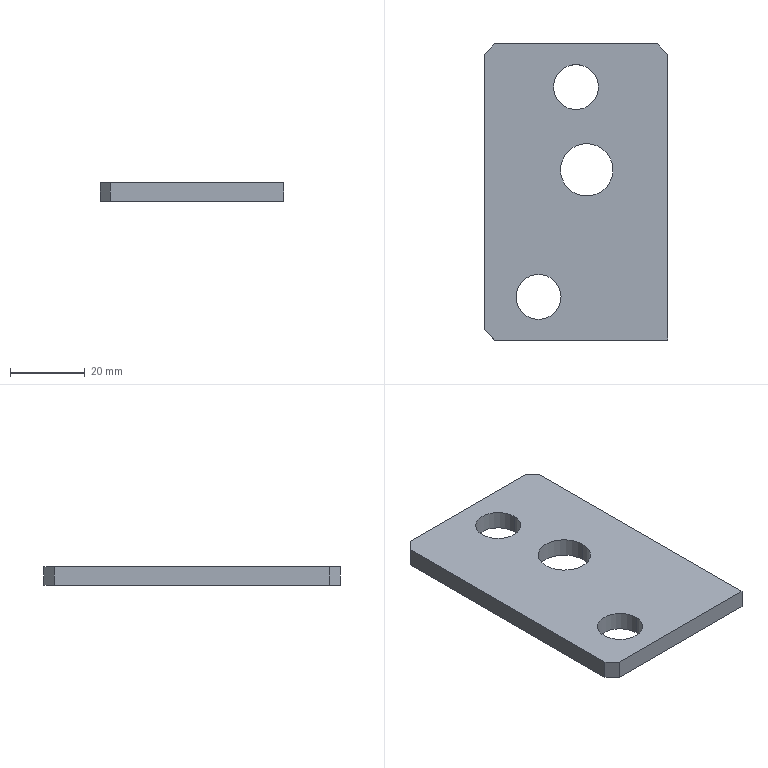Part | STEP file | 1_id646_x_t | 1 solid | 15 faces | box 49 x 79 x 5 mm | volume 17399 mm3 | plane 9 | cylinder 6 | commonest cylinder face diameters 12 x4 14 x2
STEP:
#1=CARTESIAN_POINT('',(0.,0.,0.));
#2=DIRECTION('',(0.,0.,1.));
#3=DIRECTION('',(1.,0.,0.));
#4=AXIS2_PLACEMENT_3D('',#1,#2,#3);
#5=CARTESIAN_POINT('',(168.943,211.1,-38.1));
#6=VERTEX_POINT('',#5);
#7=CARTESIAN_POINT('',(168.943,211.1,-43.1));
#8=VERTEX_POINT('',#7);
#9=CARTESIAN_POINT('',(168.943,211.1,-38.1));
#10=DIRECTION('',(0.,0.,-1.));
#11=VECTOR('',#10,1.);
#12=LINE('',#9,#11);
#13=CARTESIAN_POINT('',(149.775,211.1,-43.1));
#14=DIRECTION('',(0.,1.,0.));
#15=DIRECTION('',(0.,0.,-1.));
#16=AXIS2_PLACEMENT_3D('',#13,#14,#15);
#17=PLANE('',#16);
#18=CARTESIAN_POINT('',(-5.,-19.168));
#19=DIRECTION('',(1.,0.));
#20=VECTOR('',#19,1.);
#21=LINE('',#18,#20);
#22=(GEOMETRIC_REPRESENTATION_CONTEXT(2)PARAMETRIC_REPRESENTATION_CONTEXT()REPRESENTATION_CONTEXT('',''));
#23=DEFINITIONAL_REPRESENTATION('',(#21),#22);
#24=PCURVE('',#17,#23);
#25=CARTESIAN_POINT('',(173.659,206.384,-43.1));
#26=DIRECTION('',(-0.7071,-0.7071,0.));
#27=DIRECTION('',(-0.7071,0.7071,0.));
#28=AXIS2_PLACEMENT_3D('',#25,#26,#27);
#29=PLANE('',#28);
#30=CARTESIAN_POINT('',(6.67,-5.));
#31=DIRECTION('',(0.,1.));
#32=VECTOR('',#31,1.);
#33=LINE('',#30,#32);
#34=(GEOMETRIC_REPRESENTATION_CONTEXT(2)PARAMETRIC_REPRESENTATION_CONTEXT()REPRESENTATION_CONTEXT('',''));
#35=DEFINITIONAL_REPRESENTATION('',(#33),#34);
#36=PCURVE('',#29,#35);
#37=SURFACE_CURVE('',#12,(#24,#36),.PCURVE_S1.);
#38=EDGE_CURVE('',#6,#8,#37,.T.);
#39=ORIENTED_EDGE('',*,*,#38,.T.);
#40=CARTESIAN_POINT('',(125.357,211.1,-43.1));
#41=VERTEX_POINT('',#40);
#42=CARTESIAN_POINT('',(125.357,211.1,-43.1));
#43=DIRECTION('',(1.,0.,0.));
#44=VECTOR('',#43,1.);
#45=LINE('',#42,#44);
#46=CARTESIAN_POINT('',(0.,24.418));
#47=DIRECTION('',(0.,-1.));
#48=VECTOR('',#47,1.);
#49=LINE('',#46,#48);
#50=(GEOMETRIC_REPRESENTATION_CONTEXT(2)PARAMETRIC_REPRESENTATION_CONTEXT()REPRESENTATION_CONTEXT('',''));
#51=DEFINITIONAL_REPRESENTATION('',(#49),#50);
#52=PCURVE('',#17,#51);
#53=CARTESIAN_POINT('',(149.775,177.5,-43.1));
#54=DIRECTION('',(0.,0.,-1.));
#55=DIRECTION('',(-1.,0.,0.));
#56=AXIS2_PLACEMENT_3D('',#53,#54,#55);
#57=PLANE('',#56);
#58=CARTESIAN_POINT('',(24.418,33.6));
#59=DIRECTION('',(-1.,0.));
#60=VECTOR('',#59,1.);
#61=LINE('',#58,#60);
#62=(GEOMETRIC_REPRESENTATION_CONTEXT(2)PARAMETRIC_REPRESENTATION_CONTEXT()REPRESENTATION_CONTEXT('',''));
#63=DEFINITIONAL_REPRESENTATION('',(#61),#62);
#64=PCURVE('',#57,#63);
#65=SURFACE_CURVE('',#45,(#52,#64),.PCURVE_S1.);
#66=EDGE_CURVE('',#41,#8,#65,.T.);
#67=ORIENTED_EDGE('',*,*,#66,.F.);
#68=CARTESIAN_POINT('',(125.357,211.1,-38.1));
#69=VERTEX_POINT('',#68);
#70=CARTESIAN_POINT('',(125.357,211.1,-38.1));
#71=DIRECTION('',(0.,0.,-1.));
#72=VECTOR('',#71,1.);
#73=LINE('',#70,#72);
#74=CARTESIAN_POINT('',(-5.,24.418));
#75=DIRECTION('',(1.,0.));
#76=VECTOR('',#75,1.);
#77=LINE('',#74,#76);
#78=(GEOMETRIC_REPRESENTATION_CONTEXT(2)PARAMETRIC_REPRESENTATION_CONTEXT()REPRESENTATION_CONTEXT('',''));
#79=DEFINITIONAL_REPRESENTATION('',(#77),#78);
#80=PCURVE('',#17,#79);
#81=CARTESIAN_POINT('',(125.579,211.321,-43.1));
#82=DIRECTION('',(0.7071,-0.7071,0.));
#83=DIRECTION('',(-0.7071,-0.7071,0.));
#84=AXIS2_PLACEMENT_3D('',#81,#82,#83);
#85=PLANE('',#84);
#86=CARTESIAN_POINT('',(0.3132,-5.));
#87=DIRECTION('',(0.,1.));
#88=VECTOR('',#87,1.);
#89=LINE('',#86,#88);
#90=(GEOMETRIC_REPRESENTATION_CONTEXT(2)PARAMETRIC_REPRESENTATION_CONTEXT()REPRESENTATION_CONTEXT('',''));
#91=DEFINITIONAL_REPRESENTATION('',(#89),#90);
#92=PCURVE('',#85,#91);
#93=SURFACE_CURVE('',#73,(#80,#92),.PCURVE_S1.);
#94=EDGE_CURVE('',#69,#41,#93,.T.);
#95=ORIENTED_EDGE('',*,*,#94,.F.);
#96=CARTESIAN_POINT('',(125.357,211.1,-38.1));
#97=DIRECTION('',(1.,0.,0.));
#98=VECTOR('',#97,1.);
#99=LINE('',#96,#98);
#100=CARTESIAN_POINT('',(-5.,24.418));
#101=DIRECTION('',(0.,-1.));
#102=VECTOR('',#101,1.);
#103=LINE('',#100,#102);
#104=(GEOMETRIC_REPRESENTATION_CONTEXT(2)PARAMETRIC_REPRESENTATION_CONTEXT()REPRESENTATION_CONTEXT('',''));
#105=DEFINITIONAL_REPRESENTATION('',(#103),#104);
#106=PCURVE('',#17,#105);
#107=CARTESIAN_POINT('',(149.775,177.5,-38.1));
#108=DIRECTION('',(0.,0.,-1.));
#109=DIRECTION('',(-1.,0.,0.));
#110=AXIS2_PLACEMENT_3D('',#107,#108,#109);
#111=PLANE('',#110);
#112=CARTESIAN_POINT('',(24.418,33.6));
#113=DIRECTION('',(-1.,0.));
#114=VECTOR('',#113,1.);
#115=LINE('',#112,#114);
#116=(GEOMETRIC_REPRESENTATION_CONTEXT(2)PARAMETRIC_REPRESENTATION_CONTEXT()REPRESENTATION_CONTEXT('',''));
#117=DEFINITIONAL_REPRESENTATION('',(#115),#116);
#118=PCURVE('',#111,#117);
#119=SURFACE_CURVE('',#99,(#106,#118),.PCURVE_S1.);
#120=EDGE_CURVE('',#69,#6,#119,.T.);
#121=ORIENTED_EDGE('',*,*,#120,.T.);
#122=EDGE_LOOP('',(#39,#67,#95,#121));
#123=FACE_BOUND('',#122,.T.);
#124=ADVANCED_FACE('',(#123),#17,.T.);
#125=CARTESIAN_POINT('',(122.65,208.393,-38.1));
#126=VERTEX_POINT('',#125);
#127=CARTESIAN_POINT('',(125.357,211.1,-38.1));
#128=DIRECTION('',(-0.7071,-0.7071,0.));
#129=VECTOR('',#128,1.);
#130=LINE('',#127,#129);
#131=CARTESIAN_POINT('',(24.418,33.6));
#132=DIRECTION('',(0.7071,-0.7071));
#133=VECTOR('',#132,1.);
#134=LINE('',#131,#133);
#135=(GEOMETRIC_REPRESENTATION_CONTEXT(2)PARAMETRIC_REPRESENTATION_CONTEXT()REPRESENTATION_CONTEXT('',''));
#136=DEFINITIONAL_REPRESENTATION('',(#134),#135);
#137=PCURVE('',#111,#136);
#138=CARTESIAN_POINT('',(0.3132,-5.));
#139=DIRECTION('',(1.,0.));
#140=VECTOR('',#139,1.);
#141=LINE('',#138,#140);
#142=(GEOMETRIC_REPRESENTATION_CONTEXT(2)PARAMETRIC_REPRESENTATION_CONTEXT()REPRESENTATION_CONTEXT('',''));
#143=DEFINITIONAL_REPRESENTATION('',(#141),#142);
#144=PCURVE('',#85,#143);
#145=SURFACE_CURVE('',#130,(#137,#144),.PCURVE_S1.);
#146=EDGE_CURVE('',#69,#126,#145,.T.);
#147=ORIENTED_EDGE('',*,*,#146,.T.);
#148=CARTESIAN_POINT('',(122.65,134.807,-38.1));
#149=VERTEX_POINT('',#148);
#150=CARTESIAN_POINT('',(122.65,134.807,-38.1));
#151=DIRECTION('',(0.,1.,0.));
#152=VECTOR('',#151,1.);
#153=LINE('',#150,#152);
#154=CARTESIAN_POINT('',(27.125,-42.693));
#155=DIRECTION('',(0.,1.));
#156=VECTOR('',#155,1.);
#157=LINE('',#154,#156);
#158=(GEOMETRIC_REPRESENTATION_CONTEXT(2)PARAMETRIC_REPRESENTATION_CONTEXT()REPRESENTATION_CONTEXT('',''));
#159=DEFINITIONAL_REPRESENTATION('',(#157),#158);
#160=PCURVE('',#111,#159);
#161=CARTESIAN_POINT('',(122.65,173.5,-43.1));
#162=DIRECTION('',(-1.,0.,0.));
#163=DIRECTION('',(0.,0.,-1.));
#164=AXIS2_PLACEMENT_3D('',#161,#162,#163);
#165=PLANE('',#164);
#166=CARTESIAN_POINT('',(-5.,38.693));
#167=DIRECTION('',(0.,-1.));
#168=VECTOR('',#167,1.);
#169=LINE('',#166,#168);
#170=(GEOMETRIC_REPRESENTATION_CONTEXT(2)PARAMETRIC_REPRESENTATION_CONTEXT()REPRESENTATION_CONTEXT('',''));
#171=DEFINITIONAL_REPRESENTATION('',(#169),#170);
#172=PCURVE('',#165,#171);
#173=SURFACE_CURVE('',#153,(#160,#172),.PCURVE_S1.);
#174=EDGE_CURVE('',#149,#126,#173,.T.);
#175=ORIENTED_EDGE('',*,*,#174,.F.);
#176=CARTESIAN_POINT('',(125.357,132.1,-38.1));
#177=VERTEX_POINT('',#176);
#178=CARTESIAN_POINT('',(122.65,134.807,-38.1));
#179=DIRECTION('',(0.7071,-0.7071,0.));
#180=VECTOR('',#179,1.);
#181=LINE('',#178,#180);
#182=CARTESIAN_POINT('',(27.125,-42.693));
#183=DIRECTION('',(-0.7071,-0.7071));
#184=VECTOR('',#183,1.);
#185=LINE('',#182,#184);
#186=(GEOMETRIC_REPRESENTATION_CONTEXT(2)PARAMETRIC_REPRESENTATION_CONTEXT()REPRESENTATION_CONTEXT('',''));
#187=DEFINITIONAL_REPRESENTATION('',(#185),#186);
#188=PCURVE('',#111,#187);
#189=CARTESIAN_POINT('',(125.579,131.879,-43.1));
#190=DIRECTION('',(0.7071,0.7071,0.));
#191=DIRECTION('',(0.7071,-0.7071,0.));
#192=AXIS2_PLACEMENT_3D('',#189,#190,#191);
#193=PLANE('',#192);
#194=CARTESIAN_POINT('',(-4.142,-5.));
#195=DIRECTION('',(1.,0.));
#196=VECTOR('',#195,1.);
#197=LINE('',#194,#196);
#198=(GEOMETRIC_REPRESENTATION_CONTEXT(2)PARAMETRIC_REPRESENTATION_CONTEXT()REPRESENTATION_CONTEXT('',''));
#199=DEFINITIONAL_REPRESENTATION('',(#197),#198);
#200=PCURVE('',#193,#199);
#201=SURFACE_CURVE('',#181,(#188,#200),.PCURVE_S1.);
#202=EDGE_CURVE('',#149,#177,#201,.T.);
#203=ORIENTED_EDGE('',*,*,#202,.T.);
#204=CARTESIAN_POINT('',(171.65,132.1,-38.1));
#205=VERTEX_POINT('',#204);
#206=CARTESIAN_POINT('',(171.65,132.1,-38.1));
#207=DIRECTION('',(-1.,0.,0.));
#208=VECTOR('',#207,1.);
#209=LINE('',#206,#208);
#210=CARTESIAN_POINT('',(-21.875,-45.4));
#211=DIRECTION('',(1.,0.));
#212=VECTOR('',#211,1.);
#213=LINE('',#210,#212);
#214=(GEOMETRIC_REPRESENTATION_CONTEXT(2)PARAMETRIC_REPRESENTATION_CONTEXT()REPRESENTATION_CONTEXT('',''));
#215=DEFINITIONAL_REPRESENTATION('',(#213),#214);
#216=PCURVE('',#111,#215);
#217=CARTESIAN_POINT('',(149.775,132.1,-43.1));
#218=DIRECTION('',(0.,-1.,0.));
#219=DIRECTION('',(0.,0.,1.));
#220=AXIS2_PLACEMENT_3D('',#217,#218,#219);
#221=PLANE('',#220);
#222=CARTESIAN_POINT('',(5.,-21.875));
#223=DIRECTION('',(0.,1.));
#224=VECTOR('',#223,1.);
#225=LINE('',#222,#224);
#226=(GEOMETRIC_REPRESENTATION_CONTEXT(2)PARAMETRIC_REPRESENTATION_CONTEXT()REPRESENTATION_CONTEXT('',''));
#227=DEFINITIONAL_REPRESENTATION('',(#225),#226);
#228=PCURVE('',#221,#227);
#229=SURFACE_CURVE('',#209,(#216,#228),.PCURVE_S1.);
#230=EDGE_CURVE('',#205,#177,#229,.T.);
#231=ORIENTED_EDGE('',*,*,#230,.F.);
#232=CARTESIAN_POINT('',(171.65,208.393,-38.1));
#233=VERTEX_POINT('',#232);
#234=CARTESIAN_POINT('',(171.65,132.1,-38.1));
#235=DIRECTION('',(0.,1.,0.));
#236=VECTOR('',#235,1.);
#237=LINE('',#234,#236);
#238=CARTESIAN_POINT('',(-21.875,-45.4));
#239=DIRECTION('',(0.,1.));
#240=VECTOR('',#239,1.);
#241=LINE('',#238,#240);
#242=(GEOMETRIC_REPRESENTATION_CONTEXT(2)PARAMETRIC_REPRESENTATION_CONTEXT()REPRESENTATION_CONTEXT('',''));
#243=DEFINITIONAL_REPRESENTATION('',(#241),#242);
#244=PCURVE('',#111,#243);
#245=CARTESIAN_POINT('',(171.65,177.5,-43.1));
#246=DIRECTION('',(-1.,0.,0.));
#247=DIRECTION('',(0.,0.,-1.));
#248=AXIS2_PLACEMENT_3D('',#245,#246,#247);
#249=PLANE('',#248);
#250=CARTESIAN_POINT('',(-5.,45.4));
#251=DIRECTION('',(0.,-1.));
#252=VECTOR('',#251,1.);
#253=LINE('',#250,#252);
#254=(GEOMETRIC_REPRESENTATION_CONTEXT(2)PARAMETRIC_REPRESENTATION_CONTEXT()REPRESENTATION_CONTEXT('',''));
#255=DEFINITIONAL_REPRESENTATION('',(#253),#254);
#256=PCURVE('',#249,#255);
#257=SURFACE_CURVE('',#237,(#244,#256),.PCURVE_S1.);
#258=EDGE_CURVE('',#205,#233,#257,.T.);
#259=ORIENTED_EDGE('',*,*,#258,.T.);
#260=CARTESIAN_POINT('',(171.65,208.393,-38.1));
#261=DIRECTION('',(-0.7071,0.7071,0.));
#262=VECTOR('',#261,1.);
#263=LINE('',#260,#262);
#264=CARTESIAN_POINT('',(-21.875,30.893));
#265=DIRECTION('',(0.7071,0.7071));
#266=VECTOR('',#265,1.);
#267=LINE('',#264,#266);
#268=(GEOMETRIC_REPRESENTATION_CONTEXT(2)PARAMETRIC_REPRESENTATION_CONTEXT()REPRESENTATION_CONTEXT('',''));
#269=DEFINITIONAL_REPRESENTATION('',(#267),#268);
#270=PCURVE('',#111,#269);
#271=CARTESIAN_POINT('',(2.841,-5.));
#272=DIRECTION('',(1.,0.));
#273=VECTOR('',#272,1.);
#274=LINE('',#271,#273);
#275=(GEOMETRIC_REPRESENTATION_CONTEXT(2)PARAMETRIC_REPRESENTATION_CONTEXT()REPRESENTATION_CONTEXT('',''));
#276=DEFINITIONAL_REPRESENTATION('',(#274),#275);
#277=PCURVE('',#29,#276);
#278=SURFACE_CURVE('',#263,(#270,#277),.PCURVE_S1.);
#279=EDGE_CURVE('',#233,#6,#278,.T.);
#280=ORIENTED_EDGE('',*,*,#279,.T.);
#281=ORIENTED_EDGE('',*,*,#120,.F.);
#282=EDGE_LOOP('',(#147,#175,#203,#231,#259,#280,#281));
#283=FACE_BOUND('',#282,.T.);
#284=CARTESIAN_POINT('',(157.,177.5,-38.1));
#285=VERTEX_POINT('',#284);
#286=CARTESIAN_POINT('',(143.,177.5,-38.1));
#287=VERTEX_POINT('',#286);
#288=CARTESIAN_POINT('',(150.,177.5,-38.1));
#289=DIRECTION('',(0.,0.,-1.));
#290=DIRECTION('',(1.,0.,0.));
#291=AXIS2_PLACEMENT_3D('',#288,#289,#290);
#292=CIRCLE('',#291,7.);
#293=CARTESIAN_POINT('',(-0.225,-0.000000031));
#294=DIRECTION('',(-1.,0.));
#295=AXIS2_PLACEMENT_2D('',#293,#294);
#296=CIRCLE('',#295,7.);
#297=(GEOMETRIC_REPRESENTATION_CONTEXT(2)PARAMETRIC_REPRESENTATION_CONTEXT()REPRESENTATION_CONTEXT('',''));
#298=DEFINITIONAL_REPRESENTATION('',(#296),#297);
#299=PCURVE('',#111,#298);
#300=CARTESIAN_POINT('',(150.,177.5,-43.1));
#301=DIRECTION('',(0.,0.,1.));
#302=DIRECTION('',(-1.,0.,0.));
#303=AXIS2_PLACEMENT_3D('',#300,#301,#302);
#304=CYLINDRICAL_SURFACE('',#303,7.);
#305=CARTESIAN_POINT('',(3.142,5.));
#306=DIRECTION('',(-1.,0.));
#307=VECTOR('',#306,1.);
#308=LINE('',#305,#307);
#309=(GEOMETRIC_REPRESENTATION_CONTEXT(2)PARAMETRIC_REPRESENTATION_CONTEXT()REPRESENTATION_CONTEXT('',''));
#310=DEFINITIONAL_REPRESENTATION('',(#308),#309);
#311=PCURVE('',#304,#310);
#312=SURFACE_CURVE('',#292,(#299,#311),.PCURVE_S1.);
#313=EDGE_CURVE('',#285,#287,#312,.T.);
#314=ORIENTED_EDGE('',*,*,#313,.T.);
#315=CARTESIAN_POINT('',(150.,177.5,-38.1));
#316=DIRECTION('',(0.,0.,-1.));
#317=DIRECTION('',(-1.,0.,0.));
#318=AXIS2_PLACEMENT_3D('',#315,#316,#317);
#319=CIRCLE('',#318,7.);
#320=CARTESIAN_POINT('',(-0.225,-0.000000031));
#321=DIRECTION('',(1.,0.));
#322=AXIS2_PLACEMENT_2D('',#320,#321);
#323=CIRCLE('',#322,7.);
#324=(GEOMETRIC_REPRESENTATION_CONTEXT(2)PARAMETRIC_REPRESENTATION_CONTEXT()REPRESENTATION_CONTEXT('',''));
#325=DEFINITIONAL_REPRESENTATION('',(#323),#324);
#326=PCURVE('',#111,#325);
#327=CARTESIAN_POINT('',(150.,177.5,-43.1));
#328=DIRECTION('',(0.,0.,1.));
#329=DIRECTION('',(-1.,0.,0.));
#330=AXIS2_PLACEMENT_3D('',#327,#328,#329);
#331=CYLINDRICAL_SURFACE('',#330,7.);
#332=CARTESIAN_POINT('',(6.283,5.));
#333=DIRECTION('',(-1.,0.));
#334=VECTOR('',#333,1.);
#335=LINE('',#332,#334);
#336=(GEOMETRIC_REPRESENTATION_CONTEXT(2)PARAMETRIC_REPRESENTATION_CONTEXT()REPRESENTATION_CONTEXT('',''));
#337=DEFINITIONAL_REPRESENTATION('',(#335),#336);
#338=PCURVE('',#331,#337);
#339=SURFACE_CURVE('',#319,(#326,#338),.PCURVE_S1.);
#340=EDGE_CURVE('',#287,#285,#339,.T.);
#341=ORIENTED_EDGE('',*,*,#340,.T.);
#342=EDGE_LOOP('',(#314,#341));
#343=FACE_BOUND('',#342,.T.);
#344=CARTESIAN_POINT('',(143.15,143.6,-38.1));
#345=VERTEX_POINT('',#344);
#346=CARTESIAN_POINT('',(131.15,143.6,-38.1));
#347=VERTEX_POINT('',#346);
#348=CARTESIAN_POINT('',(137.15,143.6,-38.1));
#349=DIRECTION('',(0.,0.,-1.));
#350=DIRECTION('',(1.,0.,0.));
#351=AXIS2_PLACEMENT_3D('',#348,#349,#350);
#352=CIRCLE('',#351,6.);
#353=CARTESIAN_POINT('',(12.625,-33.9));
#354=DIRECTION('',(-1.,0.));
#355=AXIS2_PLACEMENT_2D('',#353,#354);
#356=CIRCLE('',#355,6.);
#357=(GEOMETRIC_REPRESENTATION_CONTEXT(2)PARAMETRIC_REPRESENTATION_CONTEXT()REPRESENTATION_CONTEXT('',''));
#358=DEFINITIONAL_REPRESENTATION('',(#356),#357);
#359=PCURVE('',#111,#358);
#360=CARTESIAN_POINT('',(137.15,143.6,-43.1));
#361=DIRECTION('',(0.,0.,1.));
#362=DIRECTION('',(-1.,0.,0.));
#363=AXIS2_PLACEMENT_3D('',#360,#361,#362);
#364=CYLINDRICAL_SURFACE('',#363,6.);
#365=CARTESIAN_POINT('',(3.142,5.));
#366=DIRECTION('',(-1.,0.));
#367=VECTOR('',#366,1.);
#368=LINE('',#365,#367);
#369=(GEOMETRIC_REPRESENTATION_CONTEXT(2)PARAMETRIC_REPRESENTATION_CONTEXT()REPRESENTATION_CONTEXT('',''));
#370=DEFINITIONAL_REPRESENTATION('',(#368),#369);
#371=PCURVE('',#364,#370);
#372=SURFACE_CURVE('',#352,(#359,#371),.PCURVE_S1.);
#373=EDGE_CURVE('',#345,#347,#372,.T.);
#374=ORIENTED_EDGE('',*,*,#373,.T.);
#375=CARTESIAN_POINT('',(137.15,143.6,-38.1));
#376=DIRECTION('',(0.,0.,-1.));
#377=DIRECTION('',(-1.,0.,0.));
#378=AXIS2_PLACEMENT_3D('',#375,#376,#377);
#379=CIRCLE('',#378,6.);
#380=CARTESIAN_POINT('',(12.625,-33.9));
#381=DIRECTION('',(1.,0.));
#382=AXIS2_PLACEMENT_2D('',#380,#381);
#383=CIRCLE('',#382,6.);
#384=(GEOMETRIC_REPRESENTATION_CONTEXT(2)PARAMETRIC_REPRESENTATION_CONTEXT()REPRESENTATION_CONTEXT('',''));
#385=DEFINITIONAL_REPRESENTATION('',(#383),#384);
#386=PCURVE('',#111,#385);
#387=CARTESIAN_POINT('',(137.15,143.6,-43.1));
#388=DIRECTION('',(0.,0.,1.));
#389=DIRECTION('',(-1.,0.,0.));
#390=AXIS2_PLACEMENT_3D('',#387,#388,#389);
#391=CYLINDRICAL_SURFACE('',#390,6.);
#392=CARTESIAN_POINT('',(6.283,5.));
#393=DIRECTION('',(-1.,0.));
#394=VECTOR('',#393,1.);
#395=LINE('',#392,#394);
#396=(GEOMETRIC_REPRESENTATION_CONTEXT(2)PARAMETRIC_REPRESENTATION_CONTEXT()REPRESENTATION_CONTEXT('',''));
#397=DEFINITIONAL_REPRESENTATION('',(#395),#396);
#398=PCURVE('',#391,#397);
#399=SURFACE_CURVE('',#379,(#386,#398),.PCURVE_S1.);
#400=EDGE_CURVE('',#347,#345,#399,.T.);
#401=ORIENTED_EDGE('',*,*,#400,.T.);
#402=EDGE_LOOP('',(#374,#401));
#403=FACE_BOUND('',#402,.T.);
#404=CARTESIAN_POINT('',(153.15,199.6,-38.1));
#405=VERTEX_POINT('',#404);
#406=CARTESIAN_POINT('',(141.15,199.6,-38.1));
#407=VERTEX_POINT('',#406);
#408=CARTESIAN_POINT('',(147.15,199.6,-38.1));
#409=DIRECTION('',(0.,0.,-1.));
#410=DIRECTION('',(1.,0.,0.));
#411=AXIS2_PLACEMENT_3D('',#408,#409,#410);
#412=CIRCLE('',#411,6.);
#413=CARTESIAN_POINT('',(2.625,22.1));
#414=DIRECTION('',(-1.,0.));
#415=AXIS2_PLACEMENT_2D('',#413,#414);
#416=CIRCLE('',#415,6.);
#417=(GEOMETRIC_REPRESENTATION_CONTEXT(2)PARAMETRIC_REPRESENTATION_CONTEXT()REPRESENTATION_CONTEXT('',''));
#418=DEFINITIONAL_REPRESENTATION('',(#416),#417);
#419=PCURVE('',#111,#418);
#420=CARTESIAN_POINT('',(147.15,199.6,-43.1));
#421=DIRECTION('',(0.,0.,1.));
#422=DIRECTION('',(-1.,0.,0.));
#423=AXIS2_PLACEMENT_3D('',#420,#421,#422);
#424=CYLINDRICAL_SURFACE('',#423,6.);
#425=CARTESIAN_POINT('',(3.142,5.));
#426=DIRECTION('',(-1.,0.));
#427=VECTOR('',#426,1.);
#428=LINE('',#425,#427);
#429=(GEOMETRIC_REPRESENTATION_CONTEXT(2)PARAMETRIC_REPRESENTATION_CONTEXT()REPRESENTATION_CONTEXT('',''));
#430=DEFINITIONAL_REPRESENTATION('',(#428),#429);
#431=PCURVE('',#424,#430);
#432=SURFACE_CURVE('',#412,(#419,#431),.PCURVE_S1.);
#433=EDGE_CURVE('',#405,#407,#432,.T.);
#434=ORIENTED_EDGE('',*,*,#433,.T.);
#435=CARTESIAN_POINT('',(147.15,199.6,-38.1));
#436=DIRECTION('',(0.,0.,-1.));
#437=DIRECTION('',(-1.,0.,0.));
#438=AXIS2_PLACEMENT_3D('',#435,#436,#437);
#439=CIRCLE('',#438,6.);
#440=CARTESIAN_POINT('',(2.625,22.1));
#441=DIRECTION('',(1.,0.));
#442=AXIS2_PLACEMENT_2D('',#440,#441);
#443=CIRCLE('',#442,6.);
#444=(GEOMETRIC_REPRESENTATION_CONTEXT(2)PARAMETRIC_REPRESENTATION_CONTEXT()REPRESENTATION_CONTEXT('',''));
#445=DEFINITIONAL_REPRESENTATION('',(#443),#444);
#446=PCURVE('',#111,#445);
#447=CARTESIAN_POINT('',(147.15,199.6,-43.1));
#448=DIRECTION('',(0.,0.,1.));
#449=DIRECTION('',(-1.,0.,0.));
#450=AXIS2_PLACEMENT_3D('',#447,#448,#449);
#451=CYLINDRICAL_SURFACE('',#450,6.);
#452=CARTESIAN_POINT('',(6.283,5.));
#453=DIRECTION('',(-1.,0.));
#454=VECTOR('',#453,1.);
#455=LINE('',#452,#454);
#456=(GEOMETRIC_REPRESENTATION_CONTEXT(2)PARAMETRIC_REPRESENTATION_CONTEXT()REPRESENTATION_CONTEXT('',''));
#457=DEFINITIONAL_REPRESENTATION('',(#455),#456);
#458=PCURVE('',#451,#457);
#459=SURFACE_CURVE('',#439,(#446,#458),.PCURVE_S1.);
#460=EDGE_CURVE('',#407,#405,#459,.T.);
#461=ORIENTED_EDGE('',*,*,#460,.T.);
#462=EDGE_LOOP('',(#434,#461));
#463=FACE_BOUND('',#462,.T.);
#464=ADVANCED_FACE('',(#283,#343,#403,#463),#111,.F.);
#465=CARTESIAN_POINT('',(157.,177.5,-43.1));
#466=VERTEX_POINT('',#465);
#467=CARTESIAN_POINT('',(143.,177.5,-43.1));
#468=VERTEX_POINT('',#467);
#469=CARTESIAN_POINT('',(150.,177.5,-43.1));
#470=DIRECTION('',(0.,0.,1.));
#471=DIRECTION('',(1.,0.,0.));
#472=AXIS2_PLACEMENT_3D('',#469,#470,#471);
#473=CIRCLE('',#472,7.);
#474=CARTESIAN_POINT('',(3.142,0.));
#475=DIRECTION('',(1.,0.));
#476=VECTOR('',#475,1.);
#477=LINE('',#474,#476);
#478=(GEOMETRIC_REPRESENTATION_CONTEXT(2)PARAMETRIC_REPRESENTATION_CONTEXT()REPRESENTATION_CONTEXT('',''));
#479=DEFINITIONAL_REPRESENTATION('',(#477),#478);
#480=PCURVE('',#331,#479);
#481=CARTESIAN_POINT('',(-7.225,-0.000000031));
#482=CARTESIAN_POINT('',(-7.225,12.124));
#483=CARTESIAN_POINT('',(3.275,6.062));
#484=CARTESIAN_POINT('',(13.775,-0.000000031));
#485=CARTESIAN_POINT('',(3.275,-6.062));
#486=CARTESIAN_POINT('',(-7.225,-12.124));
#487=CARTESIAN_POINT('',(-7.225,-0.000000031));
#488=(BOUNDED_CURVE()B_SPLINE_CURVE(2,(#481,#482,#483,#484,#485,#486,#487),.UNSPECIFIED.,.T.,.F.)B_SPLINE_CURVE_WITH_KNOTS((1,2,2,2,2,1),(-2.094,0.,2.094,4.189,6.283,8.378),.UNSPECIFIED.)CURVE()GEOMETRIC_REPRESENTATION_ITEM()RATIONAL_B_SPLINE_CURVE((1.,0.5,1.,0.5,1.,0.5,1.))REPRESENTATION_ITEM(''));
#489=(GEOMETRIC_REPRESENTATION_CONTEXT(2)PARAMETRIC_REPRESENTATION_CONTEXT()REPRESENTATION_CONTEXT('',''));
#490=DEFINITIONAL_REPRESENTATION('',(#488),#489);
#491=PCURVE('',#57,#490);
#492=SURFACE_CURVE('',#473,(#480,#491),.PCURVE_S1.);
#493=EDGE_CURVE('',#466,#468,#492,.T.);
#494=ORIENTED_EDGE('',*,*,#493,.T.);
#495=CARTESIAN_POINT('',(143.,177.5,-43.1));
#496=DIRECTION('',(0.,0.,1.));
#497=VECTOR('',#496,1.);
#498=LINE('',#495,#497);
#499=CARTESIAN_POINT('',(6.283,0.));
#500=DIRECTION('',(0.,1.));
#501=VECTOR('',#500,1.);
#502=LINE('',#499,#501);
#503=(GEOMETRIC_REPRESENTATION_CONTEXT(2)PARAMETRIC_REPRESENTATION_CONTEXT()REPRESENTATION_CONTEXT('',''));
#504=DEFINITIONAL_REPRESENTATION('',(#502),#503);
#505=PCURVE('',#331,#504);
#506=CARTESIAN_POINT('',(0.,0.));
#507=DIRECTION('',(0.,1.));
#508=VECTOR('',#507,1.);
#509=LINE('',#506,#508);
#510=(GEOMETRIC_REPRESENTATION_CONTEXT(2)PARAMETRIC_REPRESENTATION_CONTEXT()REPRESENTATION_CONTEXT('',''));
#511=DEFINITIONAL_REPRESENTATION('',(#509),#510);
#512=PCURVE('',#304,#511);
#513=SURFACE_CURVE('',#498,(#505,#512),.PCURVE_S1.);
#514=EDGE_CURVE('',#468,#287,#513,.T.);
#515=ORIENTED_EDGE('',*,*,#514,.T.);
#516=ORIENTED_EDGE('',*,*,#340,.T.);
#517=CARTESIAN_POINT('',(157.,177.5,-43.1));
#518=DIRECTION('',(0.,0.,-1.));
#519=VECTOR('',#518,1.);
#520=LINE('',#517,#519);
#521=CARTESIAN_POINT('',(3.142,0.));
#522=DIRECTION('',(0.,-1.));
#523=VECTOR('',#522,1.);
#524=LINE('',#521,#523);
#525=(GEOMETRIC_REPRESENTATION_CONTEXT(2)PARAMETRIC_REPRESENTATION_CONTEXT()REPRESENTATION_CONTEXT('',''));
#526=DEFINITIONAL_REPRESENTATION('',(#524),#525);
#527=PCURVE('',#331,#526);
#528=CARTESIAN_POINT('',(3.142,0.));
#529=DIRECTION('',(0.,-1.));
#530=VECTOR('',#529,1.);
#531=LINE('',#528,#530);
#532=(GEOMETRIC_REPRESENTATION_CONTEXT(2)PARAMETRIC_REPRESENTATION_CONTEXT()REPRESENTATION_CONTEXT('',''));
#533=DEFINITIONAL_REPRESENTATION('',(#531),#532);
#534=PCURVE('',#304,#533);
#535=SURFACE_CURVE('',#520,(#527,#534),.PCURVE_S1.);
#536=EDGE_CURVE('',#285,#466,#535,.T.);
#537=ORIENTED_EDGE('',*,*,#536,.T.);
#538=EDGE_LOOP('',(#494,#515,#516,#537));
#539=FACE_BOUND('',#538,.F.);
#540=ADVANCED_FACE('',(#539),#331,.F.);
#541=CARTESIAN_POINT('',(171.65,208.393,-43.1));
#542=VERTEX_POINT('',#541);
#543=CARTESIAN_POINT('',(168.943,211.1,-43.1));
#544=DIRECTION('',(0.7071,-0.7071,0.));
#545=VECTOR('',#544,1.);
#546=LINE('',#543,#545);
#547=CARTESIAN_POINT('',(-19.168,33.6));
#548=DIRECTION('',(-0.7071,-0.7071));
#549=VECTOR('',#548,1.);
#550=LINE('',#547,#549);
#551=(GEOMETRIC_REPRESENTATION_CONTEXT(2)PARAMETRIC_REPRESENTATION_CONTEXT()REPRESENTATION_CONTEXT('',''));
#552=DEFINITIONAL_REPRESENTATION('',(#550),#551);
#553=PCURVE('',#57,#552);
#554=CARTESIAN_POINT('',(6.67,0.));
#555=DIRECTION('',(-1.,0.));
#556=VECTOR('',#555,1.);
#557=LINE('',#554,#556);
#558=(GEOMETRIC_REPRESENTATION_CONTEXT(2)PARAMETRIC_REPRESENTATION_CONTEXT()REPRESENTATION_CONTEXT('',''));
#559=DEFINITIONAL_REPRESENTATION('',(#557),#558);
#560=PCURVE('',#29,#559);
#561=SURFACE_CURVE('',#546,(#553,#560),.PCURVE_S1.);
#562=EDGE_CURVE('',#8,#542,#561,.T.);
#563=ORIENTED_EDGE('',*,*,#562,.T.);
#564=CARTESIAN_POINT('',(171.65,132.1,-43.1));
#565=VERTEX_POINT('',#564);
#566=CARTESIAN_POINT('',(171.65,132.1,-43.1));
#567=DIRECTION('',(0.,1.,0.));
#568=VECTOR('',#567,1.);
#569=LINE('',#566,#568);
#570=CARTESIAN_POINT('',(-21.875,-45.4));
#571=DIRECTION('',(0.,1.));
#572=VECTOR('',#571,1.);
#573=LINE('',#570,#572);
#574=(GEOMETRIC_REPRESENTATION_CONTEXT(2)PARAMETRIC_REPRESENTATION_CONTEXT()REPRESENTATION_CONTEXT('',''));
#575=DEFINITIONAL_REPRESENTATION('',(#573),#574);
#576=PCURVE('',#57,#575);
#577=CARTESIAN_POINT('',(0.,45.4));
#578=DIRECTION('',(0.,-1.));
#579=VECTOR('',#578,1.);
#580=LINE('',#577,#579);
#581=(GEOMETRIC_REPRESENTATION_CONTEXT(2)PARAMETRIC_REPRESENTATION_CONTEXT()REPRESENTATION_CONTEXT('',''));
#582=DEFINITIONAL_REPRESENTATION('',(#580),#581);
#583=PCURVE('',#249,#582);
#584=SURFACE_CURVE('',#569,(#576,#583),.PCURVE_S1.);
#585=EDGE_CURVE('',#565,#542,#584,.T.);
#586=ORIENTED_EDGE('',*,*,#585,.F.);
#587=CARTESIAN_POINT('',(125.357,132.1,-43.1));
#588=VERTEX_POINT('',#587);
#589=CARTESIAN_POINT('',(171.65,132.1,-43.1));
#590=DIRECTION('',(-1.,0.,0.));
#591=VECTOR('',#590,1.);
#592=LINE('',#589,#591);
#593=CARTESIAN_POINT('',(-21.875,-45.4));
#594=DIRECTION('',(1.,0.));
#595=VECTOR('',#594,1.);
#596=LINE('',#593,#595);
#597=(GEOMETRIC_REPRESENTATION_CONTEXT(2)PARAMETRIC_REPRESENTATION_CONTEXT()REPRESENTATION_CONTEXT('',''));
#598=DEFINITIONAL_REPRESENTATION('',(#596),#597);
#599=PCURVE('',#57,#598);
#600=CARTESIAN_POINT('',(0.,-21.875));
#601=DIRECTION('',(0.,1.));
#602=VECTOR('',#601,1.);
#603=LINE('',#600,#602);
#604=(GEOMETRIC_REPRESENTATION_CONTEXT(2)PARAMETRIC_REPRESENTATION_CONTEXT()REPRESENTATION_CONTEXT('',''));
#605=DEFINITIONAL_REPRESENTATION('',(#603),#604);
#606=PCURVE('',#221,#605);
#607=SURFACE_CURVE('',#592,(#599,#606),.PCURVE_S1.);
#608=EDGE_CURVE('',#565,#588,#607,.T.);
#609=ORIENTED_EDGE('',*,*,#608,.T.);
#610=CARTESIAN_POINT('',(122.65,134.807,-43.1));
#611=VERTEX_POINT('',#610);
#612=CARTESIAN_POINT('',(125.357,132.1,-43.1));
#613=DIRECTION('',(-0.7071,0.7071,0.));
#614=VECTOR('',#613,1.);
#615=LINE('',#612,#614);
#616=CARTESIAN_POINT('',(24.418,-45.4));
#617=DIRECTION('',(0.7071,0.7071));
#618=VECTOR('',#617,1.);
#619=LINE('',#616,#618);
#620=(GEOMETRIC_REPRESENTATION_CONTEXT(2)PARAMETRIC_REPRESENTATION_CONTEXT()REPRESENTATION_CONTEXT('',''));
#621=DEFINITIONAL_REPRESENTATION('',(#619),#620);
#622=PCURVE('',#57,#621);
#623=CARTESIAN_POINT('',(-0.3132,0.));
#624=DIRECTION('',(-1.,0.));
#625=VECTOR('',#624,1.);
#626=LINE('',#623,#625);
#627=(GEOMETRIC_REPRESENTATION_CONTEXT(2)PARAMETRIC_REPRESENTATION_CONTEXT()REPRESENTATION_CONTEXT('',''));
#628=DEFINITIONAL_REPRESENTATION('',(#626),#627);
#629=PCURVE('',#193,#628);
#630=SURFACE_CURVE('',#615,(#622,#629),.PCURVE_S1.);
#631=EDGE_CURVE('',#588,#611,#630,.T.);
#632=ORIENTED_EDGE('',*,*,#631,.T.);
#633=CARTESIAN_POINT('',(122.65,208.393,-43.1));
#634=VERTEX_POINT('',#633);
#635=CARTESIAN_POINT('',(122.65,134.807,-43.1));
#636=DIRECTION('',(0.,1.,0.));
#637=VECTOR('',#636,1.);
#638=LINE('',#635,#637);
#639=CARTESIAN_POINT('',(27.125,-42.693));
#640=DIRECTION('',(0.,1.));
#641=VECTOR('',#640,1.);
#642=LINE('',#639,#641);
#643=(GEOMETRIC_REPRESENTATION_CONTEXT(2)PARAMETRIC_REPRESENTATION_CONTEXT()REPRESENTATION_CONTEXT('',''));
#644=DEFINITIONAL_REPRESENTATION('',(#642),#643);
#645=PCURVE('',#57,#644);
#646=CARTESIAN_POINT('',(0.,38.693));
#647=DIRECTION('',(0.,-1.));
#648=VECTOR('',#647,1.);
#649=LINE('',#646,#648);
#650=(GEOMETRIC_REPRESENTATION_CONTEXT(2)PARAMETRIC_REPRESENTATION_CONTEXT()REPRESENTATION_CONTEXT('',''));
#651=DEFINITIONAL_REPRESENTATION('',(#649),#650);
#652=PCURVE('',#165,#651);
#653=SURFACE_CURVE('',#638,(#645,#652),.PCURVE_S1.);
#654=EDGE_CURVE('',#611,#634,#653,.T.);
#655=ORIENTED_EDGE('',*,*,#654,.T.);
#656=CARTESIAN_POINT('',(122.65,208.393,-43.1));
#657=DIRECTION('',(0.7071,0.7071,0.));
#658=VECTOR('',#657,1.);
#659=LINE('',#656,#658);
#660=CARTESIAN_POINT('',(27.125,30.893));
#661=DIRECTION('',(-0.7071,0.7071));
#662=VECTOR('',#661,1.);
#663=LINE('',#660,#662);
#664=(GEOMETRIC_REPRESENTATION_CONTEXT(2)PARAMETRIC_REPRESENTATION_CONTEXT()REPRESENTATION_CONTEXT('',''));
#665=DEFINITIONAL_REPRESENTATION('',(#663),#664);
#666=PCURVE('',#57,#665);
#667=CARTESIAN_POINT('',(4.142,0.));
#668=DIRECTION('',(-1.,0.));
#669=VECTOR('',#668,1.);
#670=LINE('',#667,#669);
#671=(GEOMETRIC_REPRESENTATION_CONTEXT(2)PARAMETRIC_REPRESENTATION_CONTEXT()REPRESENTATION_CONTEXT('',''));
#672=DEFINITIONAL_REPRESENTATION('',(#670),#671);
#673=PCURVE('',#85,#672);
#674=SURFACE_CURVE('',#659,(#666,#673),.PCURVE_S1.);
#675=EDGE_CURVE('',#634,#41,#674,.T.);
#676=ORIENTED_EDGE('',*,*,#675,.T.);
#677=ORIENTED_EDGE('',*,*,#66,.T.);
#678=EDGE_LOOP('',(#563,#586,#609,#632,#655,#676,#677));
#679=FACE_BOUND('',#678,.T.);
#680=ORIENTED_EDGE('',*,*,#493,.T.);
#681=CARTESIAN_POINT('',(150.,177.5,-43.1));
#682=DIRECTION('',(0.,0.,1.));
#683=DIRECTION('',(-1.,0.,0.));
#684=AXIS2_PLACEMENT_3D('',#681,#682,#683);
#685=CIRCLE('',#684,7.);
#686=CARTESIAN_POINT('',(6.775,-0.000000031));
#687=CARTESIAN_POINT('',(6.775,-12.124));
#688=CARTESIAN_POINT('',(-3.725,-6.062));
#689=CARTESIAN_POINT('',(-14.225,-0.000000031));
#690=CARTESIAN_POINT('',(-3.725,6.062));
#691=CARTESIAN_POINT('',(6.775,12.124));
#692=CARTESIAN_POINT('',(6.775,-0.000000031));
#693=(BOUNDED_CURVE()B_SPLINE_CURVE(2,(#686,#687,#688,#689,#690,#691,#692),.UNSPECIFIED.,.T.,.F.)B_SPLINE_CURVE_WITH_KNOTS((1,2,2,2,2,1),(-2.094,0.,2.094,4.189,6.283,8.378),.UNSPECIFIED.)CURVE()GEOMETRIC_REPRESENTATION_ITEM()RATIONAL_B_SPLINE_CURVE((1.,0.5,1.,0.5,1.,0.5,1.))REPRESENTATION_ITEM(''));
#694=(GEOMETRIC_REPRESENTATION_CONTEXT(2)PARAMETRIC_REPRESENTATION_CONTEXT()REPRESENTATION_CONTEXT('',''));
#695=DEFINITIONAL_REPRESENTATION('',(#693),#694);
#696=PCURVE('',#57,#695);
#697=CARTESIAN_POINT('',(0.,0.));
#698=DIRECTION('',(1.,0.));
#699=VECTOR('',#698,1.);
#700=LINE('',#697,#699);
#701=(GEOMETRIC_REPRESENTATION_CONTEXT(2)PARAMETRIC_REPRESENTATION_CONTEXT()REPRESENTATION_CONTEXT('',''));
#702=DEFINITIONAL_REPRESENTATION('',(#700),#701);
#703=PCURVE('',#304,#702);
#704=SURFACE_CURVE('',#685,(#696,#703),.PCURVE_S1.);
#705=EDGE_CURVE('',#468,#466,#704,.T.);
#706=ORIENTED_EDGE('',*,*,#705,.T.);
#707=EDGE_LOOP('',(#680,#706));
#708=FACE_BOUND('',#707,.T.);
#709=CARTESIAN_POINT('',(143.15,143.6,-43.1));
#710=VERTEX_POINT('',#709);
#711=CARTESIAN_POINT('',(131.15,143.6,-43.1));
#712=VERTEX_POINT('',#711);
#713=CARTESIAN_POINT('',(137.15,143.6,-43.1));
#714=DIRECTION('',(0.,0.,1.));
#715=DIRECTION('',(1.,0.,0.));
#716=AXIS2_PLACEMENT_3D('',#713,#714,#715);
#717=CIRCLE('',#716,6.);
#718=CARTESIAN_POINT('',(6.625,-33.9));
#719=CARTESIAN_POINT('',(6.625,-23.508));
#720=CARTESIAN_POINT('',(15.625,-28.704));
#721=CARTESIAN_POINT('',(24.625,-33.9));
#722=CARTESIAN_POINT('',(15.625,-39.096));
#723=CARTESIAN_POINT('',(6.625,-44.292));
#724=CARTESIAN_POINT('',(6.625,-33.9));
#725=(BOUNDED_CURVE()B_SPLINE_CURVE(2,(#718,#719,#720,#721,#722,#723,#724),.UNSPECIFIED.,.T.,.F.)B_SPLINE_CURVE_WITH_KNOTS((1,2,2,2,2,1),(-2.094,0.,2.094,4.189,6.283,8.378),.UNSPECIFIED.)CURVE()GEOMETRIC_REPRESENTATION_ITEM()RATIONAL_B_SPLINE_CURVE((1.,0.5,1.,0.5,1.,0.5,1.))REPRESENTATION_ITEM(''));
#726=(GEOMETRIC_REPRESENTATION_CONTEXT(2)PARAMETRIC_REPRESENTATION_CONTEXT()REPRESENTATION_CONTEXT('',''));
#727=DEFINITIONAL_REPRESENTATION('',(#725),#726);
#728=PCURVE('',#57,#727);
#729=CARTESIAN_POINT('',(3.142,0.));
#730=DIRECTION('',(1.,0.));
#731=VECTOR('',#730,1.);
#732=LINE('',#729,#731);
#733=(GEOMETRIC_REPRESENTATION_CONTEXT(2)PARAMETRIC_REPRESENTATION_CONTEXT()REPRESENTATION_CONTEXT('',''));
#734=DEFINITIONAL_REPRESENTATION('',(#732),#733);
#735=PCURVE('',#391,#734);
#736=SURFACE_CURVE('',#717,(#728,#735),.PCURVE_S1.);
#737=EDGE_CURVE('',#710,#712,#736,.T.);
#738=ORIENTED_EDGE('',*,*,#737,.T.);
#739=CARTESIAN_POINT('',(137.15,143.6,-43.1));
#740=DIRECTION('',(0.,0.,1.));
#741=DIRECTION('',(-1.,0.,0.));
#742=AXIS2_PLACEMENT_3D('',#739,#740,#741);
#743=CIRCLE('',#742,6.);
#744=CARTESIAN_POINT('',(18.625,-33.9));
#745=CARTESIAN_POINT('',(18.625,-44.292));
#746=CARTESIAN_POINT('',(9.625,-39.096));
#747=CARTESIAN_POINT('',(0.625,-33.9));
#748=CARTESIAN_POINT('',(9.625,-28.704));
#749=CARTESIAN_POINT('',(18.625,-23.508));
#750=CARTESIAN_POINT('',(18.625,-33.9));
#751=(BOUNDED_CURVE()B_SPLINE_CURVE(2,(#744,#745,#746,#747,#748,#749,#750),.UNSPECIFIED.,.T.,.F.)B_SPLINE_CURVE_WITH_KNOTS((1,2,2,2,2,1),(-2.094,0.,2.094,4.189,6.283,8.378),.UNSPECIFIED.)CURVE()GEOMETRIC_REPRESENTATION_ITEM()RATIONAL_B_SPLINE_CURVE((1.,0.5,1.,0.5,1.,0.5,1.))REPRESENTATION_ITEM(''));
#752=(GEOMETRIC_REPRESENTATION_CONTEXT(2)PARAMETRIC_REPRESENTATION_CONTEXT()REPRESENTATION_CONTEXT('',''));
#753=DEFINITIONAL_REPRESENTATION('',(#751),#752);
#754=PCURVE('',#57,#753);
#755=CARTESIAN_POINT('',(0.,0.));
#756=DIRECTION('',(1.,0.));
#757=VECTOR('',#756,1.);
#758=LINE('',#755,#757);
#759=(GEOMETRIC_REPRESENTATION_CONTEXT(2)PARAMETRIC_REPRESENTATION_CONTEXT()REPRESENTATION_CONTEXT('',''));
#760=DEFINITIONAL_REPRESENTATION('',(#758),#759);
#761=PCURVE('',#364,#760);
#762=SURFACE_CURVE('',#743,(#754,#761),.PCURVE_S1.);
#763=EDGE_CURVE('',#712,#710,#762,.T.);
#764=ORIENTED_EDGE('',*,*,#763,.T.);
#765=EDGE_LOOP('',(#738,#764));
#766=FACE_BOUND('',#765,.T.);
#767=CARTESIAN_POINT('',(153.15,199.6,-43.1));
#768=VERTEX_POINT('',#767);
#769=CARTESIAN_POINT('',(141.15,199.6,-43.1));
#770=VERTEX_POINT('',#769);
#771=CARTESIAN_POINT('',(147.15,199.6,-43.1));
#772=DIRECTION('',(0.,0.,1.));
#773=DIRECTION('',(1.,0.,0.));
#774=AXIS2_PLACEMENT_3D('',#771,#772,#773);
#775=CIRCLE('',#774,6.);
#776=CARTESIAN_POINT('',(-3.375,22.1));
#777=CARTESIAN_POINT('',(-3.375,32.492));
#778=CARTESIAN_POINT('',(5.625,27.296));
#779=CARTESIAN_POINT('',(14.625,22.1));
#780=CARTESIAN_POINT('',(5.625,16.904));
#781=CARTESIAN_POINT('',(-3.375,11.708));
#782=CARTESIAN_POINT('',(-3.375,22.1));
#783=(BOUNDED_CURVE()B_SPLINE_CURVE(2,(#776,#777,#778,#779,#780,#781,#782),.UNSPECIFIED.,.T.,.F.)B_SPLINE_CURVE_WITH_KNOTS((1,2,2,2,2,1),(-2.094,0.,2.094,4.189,6.283,8.378),.UNSPECIFIED.)CURVE()GEOMETRIC_REPRESENTATION_ITEM()RATIONAL_B_SPLINE_CURVE((1.,0.5,1.,0.5,1.,0.5,1.))REPRESENTATION_ITEM(''));
#784=(GEOMETRIC_REPRESENTATION_CONTEXT(2)PARAMETRIC_REPRESENTATION_CONTEXT()REPRESENTATION_CONTEXT('',''));
#785=DEFINITIONAL_REPRESENTATION('',(#783),#784);
#786=PCURVE('',#57,#785);
#787=CARTESIAN_POINT('',(3.142,0.));
#788=DIRECTION('',(1.,0.));
#789=VECTOR('',#788,1.);
#790=LINE('',#787,#789);
#791=(GEOMETRIC_REPRESENTATION_CONTEXT(2)PARAMETRIC_REPRESENTATION_CONTEXT()REPRESENTATION_CONTEXT('',''));
#792=DEFINITIONAL_REPRESENTATION('',(#790),#791);
#793=PCURVE('',#451,#792);
#794=SURFACE_CURVE('',#775,(#786,#793),.PCURVE_S1.);
#795=EDGE_CURVE('',#768,#770,#794,.T.);
#796=ORIENTED_EDGE('',*,*,#795,.T.);
#797=CARTESIAN_POINT('',(147.15,199.6,-43.1));
#798=DIRECTION('',(0.,0.,1.));
#799=DIRECTION('',(-1.,0.,0.));
#800=AXIS2_PLACEMENT_3D('',#797,#798,#799);
#801=CIRCLE('',#800,6.);
#802=CARTESIAN_POINT('',(8.625,22.1));
#803=CARTESIAN_POINT('',(8.625,11.708));
#804=CARTESIAN_POINT('',(-0.375,16.904));
#805=CARTESIAN_POINT('',(-9.375,22.1));
#806=CARTESIAN_POINT('',(-0.375,27.296));
#807=CARTESIAN_POINT('',(8.625,32.492));
#808=CARTESIAN_POINT('',(8.625,22.1));
#809=(BOUNDED_CURVE()B_SPLINE_CURVE(2,(#802,#803,#804,#805,#806,#807,#808),.UNSPECIFIED.,.T.,.F.)B_SPLINE_CURVE_WITH_KNOTS((1,2,2,2,2,1),(-2.094,0.,2.094,4.189,6.283,8.378),.UNSPECIFIED.)CURVE()GEOMETRIC_REPRESENTATION_ITEM()RATIONAL_B_SPLINE_CURVE((1.,0.5,1.,0.5,1.,0.5,1.))REPRESENTATION_ITEM(''));
#810=(GEOMETRIC_REPRESENTATION_CONTEXT(2)PARAMETRIC_REPRESENTATION_CONTEXT()REPRESENTATION_CONTEXT('',''));
#811=DEFINITIONAL_REPRESENTATION('',(#809),#810);
#812=PCURVE('',#57,#811);
#813=CARTESIAN_POINT('',(0.,0.));
#814=DIRECTION('',(1.,0.));
#815=VECTOR('',#814,1.);
#816=LINE('',#813,#815);
#817=(GEOMETRIC_REPRESENTATION_CONTEXT(2)PARAMETRIC_REPRESENTATION_CONTEXT()REPRESENTATION_CONTEXT('',''));
#818=DEFINITIONAL_REPRESENTATION('',(#816),#817);
#819=PCURVE('',#424,#818);
#820=SURFACE_CURVE('',#801,(#812,#819),.PCURVE_S1.);
#821=EDGE_CURVE('',#770,#768,#820,.T.);
#822=ORIENTED_EDGE('',*,*,#821,.T.);
#823=EDGE_LOOP('',(#796,#822));
#824=FACE_BOUND('',#823,.T.);
#825=ADVANCED_FACE('',(#679,#708,#766,#824),#57,.T.);
#826=ORIENTED_EDGE('',*,*,#705,.T.);
#827=ORIENTED_EDGE('',*,*,#536,.F.);
#828=ORIENTED_EDGE('',*,*,#313,.T.);
#829=ORIENTED_EDGE('',*,*,#514,.F.);
#830=EDGE_LOOP('',(#826,#827,#828,#829));
#831=FACE_BOUND('',#830,.F.);
#832=ADVANCED_FACE('',(#831),#304,.F.);
#833=ORIENTED_EDGE('',*,*,#763,.T.);
#834=CARTESIAN_POINT('',(143.15,143.6,-43.1));
#835=DIRECTION('',(0.,0.,-1.));
#836=VECTOR('',#835,1.);
#837=LINE('',#834,#836);
#838=CARTESIAN_POINT('',(3.142,0.));
#839=DIRECTION('',(0.,-1.));
#840=VECTOR('',#839,1.);
#841=LINE('',#838,#840);
#842=(GEOMETRIC_REPRESENTATION_CONTEXT(2)PARAMETRIC_REPRESENTATION_CONTEXT()REPRESENTATION_CONTEXT('',''));
#843=DEFINITIONAL_REPRESENTATION('',(#841),#842);
#844=PCURVE('',#364,#843);
#845=CARTESIAN_POINT('',(3.142,0.));
#846=DIRECTION('',(0.,-1.));
#847=VECTOR('',#846,1.);
#848=LINE('',#845,#847);
#849=(GEOMETRIC_REPRESENTATION_CONTEXT(2)PARAMETRIC_REPRESENTATION_CONTEXT()REPRESENTATION_CONTEXT('',''));
#850=DEFINITIONAL_REPRESENTATION('',(#848),#849);
#851=PCURVE('',#391,#850);
#852=SURFACE_CURVE('',#837,(#844,#851),.PCURVE_S1.);
#853=EDGE_CURVE('',#345,#710,#852,.T.);
#854=ORIENTED_EDGE('',*,*,#853,.F.);
#855=ORIENTED_EDGE('',*,*,#373,.T.);
#856=CARTESIAN_POINT('',(131.15,143.6,-43.1));
#857=DIRECTION('',(0.,0.,1.));
#858=VECTOR('',#857,1.);
#859=LINE('',#856,#858);
#860=CARTESIAN_POINT('',(0.,0.));
#861=DIRECTION('',(0.,1.));
#862=VECTOR('',#861,1.);
#863=LINE('',#860,#862);
#864=(GEOMETRIC_REPRESENTATION_CONTEXT(2)PARAMETRIC_REPRESENTATION_CONTEXT()REPRESENTATION_CONTEXT('',''));
#865=DEFINITIONAL_REPRESENTATION('',(#863),#864);
#866=PCURVE('',#364,#865);
#867=CARTESIAN_POINT('',(6.283,0.));
#868=DIRECTION('',(0.,1.));
#869=VECTOR('',#868,1.);
#870=LINE('',#867,#869);
#871=(GEOMETRIC_REPRESENTATION_CONTEXT(2)PARAMETRIC_REPRESENTATION_CONTEXT()REPRESENTATION_CONTEXT('',''));
#872=DEFINITIONAL_REPRESENTATION('',(#870),#871);
#873=PCURVE('',#391,#872);
#874=SURFACE_CURVE('',#859,(#866,#873),.PCURVE_S1.);
#875=EDGE_CURVE('',#712,#347,#874,.T.);
#876=ORIENTED_EDGE('',*,*,#875,.F.);
#877=EDGE_LOOP('',(#833,#854,#855,#876));
#878=FACE_BOUND('',#877,.F.);
#879=ADVANCED_FACE('',(#878),#364,.F.);
#880=ORIENTED_EDGE('',*,*,#737,.T.);
#881=ORIENTED_EDGE('',*,*,#875,.T.);
#882=ORIENTED_EDGE('',*,*,#400,.T.);
#883=ORIENTED_EDGE('',*,*,#853,.T.);
#884=EDGE_LOOP('',(#880,#881,#882,#883));
#885=FACE_BOUND('',#884,.F.);
#886=ADVANCED_FACE('',(#885),#391,.F.);
#887=ORIENTED_EDGE('',*,*,#821,.T.);
#888=CARTESIAN_POINT('',(153.15,199.6,-43.1));
#889=DIRECTION('',(0.,0.,1.));
#890=VECTOR('',#889,1.);
#891=LINE('',#888,#890);
#892=CARTESIAN_POINT('',(3.142,0.));
#893=DIRECTION('',(0.,1.));
#894=VECTOR('',#893,1.);
#895=LINE('',#892,#894);
#896=(GEOMETRIC_REPRESENTATION_CONTEXT(2)PARAMETRIC_REPRESENTATION_CONTEXT()REPRESENTATION_CONTEXT('',''));
#897=DEFINITIONAL_REPRESENTATION('',(#895),#896);
#898=PCURVE('',#424,#897);
#899=CARTESIAN_POINT('',(3.142,0.));
#900=DIRECTION('',(0.,1.));
#901=VECTOR('',#900,1.);
#902=LINE('',#899,#901);
#903=(GEOMETRIC_REPRESENTATION_CONTEXT(2)PARAMETRIC_REPRESENTATION_CONTEXT()REPRESENTATION_CONTEXT('',''));
#904=DEFINITIONAL_REPRESENTATION('',(#902),#903);
#905=PCURVE('',#451,#904);
#906=SURFACE_CURVE('',#891,(#898,#905),.PCURVE_S1.);
#907=EDGE_CURVE('',#768,#405,#906,.T.);
#908=ORIENTED_EDGE('',*,*,#907,.T.);
#909=ORIENTED_EDGE('',*,*,#433,.T.);
#910=CARTESIAN_POINT('',(141.15,199.6,-43.1));
#911=DIRECTION('',(0.,0.,-1.));
#912=VECTOR('',#911,1.);
#913=LINE('',#910,#912);
#914=CARTESIAN_POINT('',(0.,0.));
#915=DIRECTION('',(0.,-1.));
#916=VECTOR('',#915,1.);
#917=LINE('',#914,#916);
#918=(GEOMETRIC_REPRESENTATION_CONTEXT(2)PARAMETRIC_REPRESENTATION_CONTEXT()REPRESENTATION_CONTEXT('',''));
#919=DEFINITIONAL_REPRESENTATION('',(#917),#918);
#920=PCURVE('',#424,#919);
#921=CARTESIAN_POINT('',(6.283,0.));
#922=DIRECTION('',(0.,-1.));
#923=VECTOR('',#922,1.);
#924=LINE('',#921,#923);
#925=(GEOMETRIC_REPRESENTATION_CONTEXT(2)PARAMETRIC_REPRESENTATION_CONTEXT()REPRESENTATION_CONTEXT('',''));
#926=DEFINITIONAL_REPRESENTATION('',(#924),#925);
#927=PCURVE('',#451,#926);
#928=SURFACE_CURVE('',#913,(#920,#927),.PCURVE_S1.);
#929=EDGE_CURVE('',#407,#770,#928,.T.);
#930=ORIENTED_EDGE('',*,*,#929,.T.);
#931=EDGE_LOOP('',(#887,#908,#909,#930));
#932=FACE_BOUND('',#931,.F.);
#933=ADVANCED_FACE('',(#932),#424,.F.);
#934=ORIENTED_EDGE('',*,*,#795,.T.);
#935=ORIENTED_EDGE('',*,*,#929,.F.);
#936=ORIENTED_EDGE('',*,*,#460,.T.);
#937=ORIENTED_EDGE('',*,*,#907,.F.);
#938=EDGE_LOOP('',(#934,#935,#936,#937));
#939=FACE_BOUND('',#938,.F.);
#940=ADVANCED_FACE('',(#939),#451,.F.);
#941=ORIENTED_EDGE('',*,*,#94,.T.);
#942=ORIENTED_EDGE('',*,*,#675,.F.);
#943=CARTESIAN_POINT('',(122.65,208.393,-38.1));
#944=DIRECTION('',(0.,0.,-1.));
#945=VECTOR('',#944,1.);
#946=LINE('',#943,#945);
#947=CARTESIAN_POINT('',(4.142,-5.));
#948=DIRECTION('',(0.,1.));
#949=VECTOR('',#948,1.);
#950=LINE('',#947,#949);
#951=(GEOMETRIC_REPRESENTATION_CONTEXT(2)PARAMETRIC_REPRESENTATION_CONTEXT()REPRESENTATION_CONTEXT('',''));
#952=DEFINITIONAL_REPRESENTATION('',(#950),#951);
#953=PCURVE('',#85,#952);
#954=CARTESIAN_POINT('',(-5.,-34.893));
#955=DIRECTION('',(1.,0.));
#956=VECTOR('',#955,1.);
#957=LINE('',#954,#956);
#958=(GEOMETRIC_REPRESENTATION_CONTEXT(2)PARAMETRIC_REPRESENTATION_CONTEXT()REPRESENTATION_CONTEXT('',''));
#959=DEFINITIONAL_REPRESENTATION('',(#957),#958);
#960=PCURVE('',#165,#959);
#961=SURFACE_CURVE('',#946,(#953,#960),.PCURVE_S1.);
#962=EDGE_CURVE('',#126,#634,#961,.T.);
#963=ORIENTED_EDGE('',*,*,#962,.F.);
#964=ORIENTED_EDGE('',*,*,#146,.F.);
#965=EDGE_LOOP('',(#941,#942,#963,#964));
#966=FACE_BOUND('',#965,.T.);
#967=ADVANCED_FACE('',(#966),#85,.F.);
#968=ORIENTED_EDGE('',*,*,#962,.T.);
#969=ORIENTED_EDGE('',*,*,#654,.F.);
#970=CARTESIAN_POINT('',(122.65,134.807,-38.1));
#971=DIRECTION('',(0.,0.,-1.));
#972=VECTOR('',#971,1.);
#973=LINE('',#970,#972);
#974=CARTESIAN_POINT('',(-5.,38.693));
#975=DIRECTION('',(1.,0.));
#976=VECTOR('',#975,1.);
#977=LINE('',#974,#976);
#978=(GEOMETRIC_REPRESENTATION_CONTEXT(2)PARAMETRIC_REPRESENTATION_CONTEXT()REPRESENTATION_CONTEXT('',''));
#979=DEFINITIONAL_REPRESENTATION('',(#977),#978);
#980=PCURVE('',#165,#979);
#981=CARTESIAN_POINT('',(-4.142,-5.));
#982=DIRECTION('',(0.,1.));
#983=VECTOR('',#982,1.);
#984=LINE('',#981,#983);
#985=(GEOMETRIC_REPRESENTATION_CONTEXT(2)PARAMETRIC_REPRESENTATION_CONTEXT()REPRESENTATION_CONTEXT('',''));
#986=DEFINITIONAL_REPRESENTATION('',(#984),#985);
#987=PCURVE('',#193,#986);
#988=SURFACE_CURVE('',#973,(#980,#987),.PCURVE_S1.);
#989=EDGE_CURVE('',#149,#611,#988,.T.);
#990=ORIENTED_EDGE('',*,*,#989,.F.);
#991=ORIENTED_EDGE('',*,*,#174,.T.);
#992=EDGE_LOOP('',(#968,#969,#990,#991));
#993=FACE_BOUND('',#992,.T.);
#994=ADVANCED_FACE('',(#993),#165,.T.);
#995=ORIENTED_EDGE('',*,*,#989,.T.);
#996=ORIENTED_EDGE('',*,*,#631,.F.);
#997=CARTESIAN_POINT('',(125.357,132.1,-38.1));
#998=DIRECTION('',(0.,0.,-1.));
#999=VECTOR('',#998,1.);
#1000=LINE('',#997,#999);
#1001=CARTESIAN_POINT('',(-0.3132,-5.));
#1002=DIRECTION('',(0.,1.));
#1003=VECTOR('',#1002,1.);
#1004=LINE('',#1001,#1003);
#1005=(GEOMETRIC_REPRESENTATION_CONTEXT(2)PARAMETRIC_REPRESENTATION_CONTEXT()REPRESENTATION_CONTEXT('',''));
#1006=DEFINITIONAL_REPRESENTATION('',(#1004),#1005);
#1007=PCURVE('',#193,#1006);
#1008=CARTESIAN_POINT('',(5.,24.418));
#1009=DIRECTION('',(-1.,0.));
#1010=VECTOR('',#1009,1.);
#1011=LINE('',#1008,#1010);
#1012=(GEOMETRIC_REPRESENTATION_CONTEXT(2)PARAMETRIC_REPRESENTATION_CONTEXT()REPRESENTATION_CONTEXT('',''));
#1013=DEFINITIONAL_REPRESENTATION('',(#1011),#1012);
#1014=PCURVE('',#221,#1013);
#1015=SURFACE_CURVE('',#1000,(#1007,#1014),.PCURVE_S1.);
#1016=EDGE_CURVE('',#177,#588,#1015,.T.);
#1017=ORIENTED_EDGE('',*,*,#1016,.F.);
#1018=ORIENTED_EDGE('',*,*,#202,.F.);
#1019=EDGE_LOOP('',(#995,#996,#1017,#1018));
#1020=FACE_BOUND('',#1019,.T.);
#1021=ADVANCED_FACE('',(#1020),#193,.F.);
#1022=ORIENTED_EDGE('',*,*,#1016,.T.);
#1023=ORIENTED_EDGE('',*,*,#608,.F.);
#1024=CARTESIAN_POINT('',(171.65,132.1,-38.1));
#1025=DIRECTION('',(0.,0.,-1.));
#1026=VECTOR('',#1025,1.);
#1027=LINE('',#1024,#1026);
#1028=CARTESIAN_POINT('',(5.,-21.875));
#1029=DIRECTION('',(-1.,0.));
#1030=VECTOR('',#1029,1.);
#1031=LINE('',#1028,#1030);
#1032=(GEOMETRIC_REPRESENTATION_CONTEXT(2)PARAMETRIC_REPRESENTATION_CONTEXT()REPRESENTATION_CONTEXT('',''));
#1033=DEFINITIONAL_REPRESENTATION('',(#1031),#1032);
#1034=PCURVE('',#221,#1033);
#1035=CARTESIAN_POINT('',(-5.,45.4));
#1036=DIRECTION('',(1.,0.));
#1037=VECTOR('',#1036,1.);
#1038=LINE('',#1035,#1037);
#1039=(GEOMETRIC_REPRESENTATION_CONTEXT(2)PARAMETRIC_REPRESENTATION_CONTEXT()REPRESENTATION_CONTEXT('',''));
#1040=DEFINITIONAL_REPRESENTATION('',(#1038),#1039);
#1041=PCURVE('',#249,#1040);
#1042=SURFACE_CURVE('',#1027,(#1034,#1041),.PCURVE_S1.);
#1043=EDGE_CURVE('',#205,#565,#1042,.T.);
#1044=ORIENTED_EDGE('',*,*,#1043,.F.);
#1045=ORIENTED_EDGE('',*,*,#230,.T.);
#1046=EDGE_LOOP('',(#1022,#1023,#1044,#1045));
#1047=FACE_BOUND('',#1046,.T.);
#1048=ADVANCED_FACE('',(#1047),#221,.T.);
#1049=ORIENTED_EDGE('',*,*,#1043,.T.);
#1050=ORIENTED_EDGE('',*,*,#585,.T.);
#1051=CARTESIAN_POINT('',(171.65,208.393,-38.1));
#1052=DIRECTION('',(0.,0.,-1.));
#1053=VECTOR('',#1052,1.);
#1054=LINE('',#1051,#1053);
#1055=CARTESIAN_POINT('',(-5.,-30.893));
#1056=DIRECTION('',(1.,0.));
#1057=VECTOR('',#1056,1.);
#1058=LINE('',#1055,#1057);
#1059=(GEOMETRIC_REPRESENTATION_CONTEXT(2)PARAMETRIC_REPRESENTATION_CONTEXT()REPRESENTATION_CONTEXT('',''));
#1060=DEFINITIONAL_REPRESENTATION('',(#1058),#1059);
#1061=PCURVE('',#249,#1060);
#1062=CARTESIAN_POINT('',(2.841,-5.));
#1063=DIRECTION('',(0.,1.));
#1064=VECTOR('',#1063,1.);
#1065=LINE('',#1062,#1064);
#1066=(GEOMETRIC_REPRESENTATION_CONTEXT(2)PARAMETRIC_REPRESENTATION_CONTEXT()REPRESENTATION_CONTEXT('',''));
#1067=DEFINITIONAL_REPRESENTATION('',(#1065),#1066);
#1068=PCURVE('',#29,#1067);
#1069=SURFACE_CURVE('',#1054,(#1061,#1068),.PCURVE_S1.);
#1070=EDGE_CURVE('',#233,#542,#1069,.T.);
#1071=ORIENTED_EDGE('',*,*,#1070,.F.);
#1072=ORIENTED_EDGE('',*,*,#258,.F.);
#1073=EDGE_LOOP('',(#1049,#1050,#1071,#1072));
#1074=FACE_BOUND('',#1073,.T.);
#1075=ADVANCED_FACE('',(#1074),#249,.F.);
#1076=ORIENTED_EDGE('',*,*,#1070,.T.);
#1077=ORIENTED_EDGE('',*,*,#562,.F.);
#1078=ORIENTED_EDGE('',*,*,#38,.F.);
#1079=ORIENTED_EDGE('',*,*,#279,.F.);
#1080=EDGE_LOOP('',(#1076,#1077,#1078,#1079));
#1081=FACE_BOUND('',#1080,.T.);
#1082=ADVANCED_FACE('',(#1081),#29,.F.);
#1083=CLOSED_SHELL('',(#124,#464,#540,#825,#832,#879,#886,#933,#940,#967,#994,#1021,#1048,#1075,#1082));
#1084=MANIFOLD_SOLID_BREP('',#1083);
#1085=(LENGTH_UNIT()NAMED_UNIT(*)SI_UNIT(.MILLI.,.METRE.));
#1086=UNCERTAINTY_MEASURE_WITH_UNIT(LENGTH_MEASURE(0.0000001),#1085,'','');
#1087=(NAMED_UNIT(*)PLANE_ANGLE_UNIT()SI_UNIT($,.RADIAN.));
#1088=(NAMED_UNIT(*)SI_UNIT($,.STERADIAN.)SOLID_ANGLE_UNIT());
#1089=(GEOMETRIC_REPRESENTATION_CONTEXT(3)GLOBAL_UNCERTAINTY_ASSIGNED_CONTEXT((#1086))GLOBAL_UNIT_ASSIGNED_CONTEXT((#1085,#1087,#1088))REPRESENTATION_CONTEXT('',''));
#1090=ADVANCED_BREP_SHAPE_REPRESENTATION('',(#4,#1084),#1089);